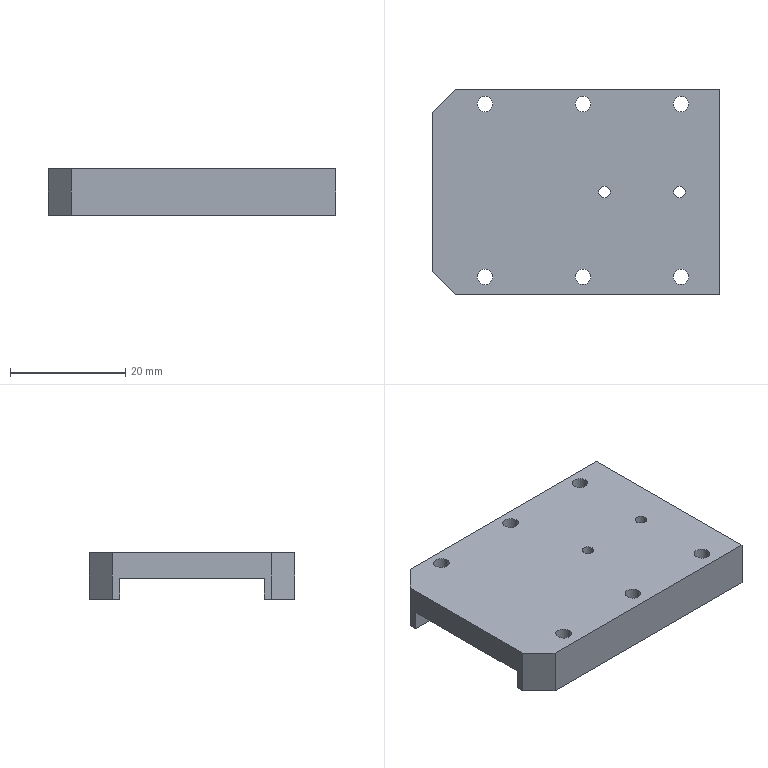Part | SolidWorks | features BaseBody 1 | 1 solid | 28 faces | box 49.9 x 35.6 x 8 mm | volume 9414 mm3 | cylinder 16 | plane 12 | commonest cylinder face diameters 2.7 x12 2 x4
STEP:
#1=CARTESIAN_POINT('',(14.5,0.,-0.5));
#2=VERTEX_POINT('',#1);
#3=CARTESIAN_POINT('',(16.5,0.,-0.5));
#4=VERTEX_POINT('',#3);
#5=CARTESIAN_POINT('',(15.5,0.,-0.5));
#6=DIRECTION('',(0.,0.,1.));
#7=DIRECTION('',(0.,-1.,0.));
#8=AXIS2_PLACEMENT_3D('',#5,#6,#7);
#9=CIRCLE('',#8,1.);
#10=EDGE_CURVE('',#2,#4,#9,.T.);
#11=ORIENTED_EDGE('',*,*,#10,.F.);
#12=CARTESIAN_POINT('',(14.5,0.,4.));
#13=VERTEX_POINT('',#12);
#14=CARTESIAN_POINT('',(14.5,0.,-4.));
#15=DIRECTION('',(0.,0.,1.));
#16=VECTOR('',#15,1000.);
#17=LINE('',#14,#16);
#18=EDGE_CURVE('',#2,#13,#17,.T.);
#19=ORIENTED_EDGE('',*,*,#18,.T.);
#20=CARTESIAN_POINT('',(16.5,0.,4.));
#21=VERTEX_POINT('',#20);
#22=CARTESIAN_POINT('',(15.5,0.,4.));
#23=DIRECTION('',(0.,0.,1.));
#24=DIRECTION('',(1.,0.,0.));
#25=AXIS2_PLACEMENT_3D('',#22,#23,#24);
#26=CIRCLE('',#25,1.);
#27=EDGE_CURVE('',#13,#21,#26,.T.);
#28=ORIENTED_EDGE('',*,*,#27,.T.);
#29=CARTESIAN_POINT('',(16.5,0.,-4.));
#30=DIRECTION('',(0.,0.,1.));
#31=VECTOR('',#30,1000.);
#32=LINE('',#29,#31);
#33=EDGE_CURVE('',#4,#21,#32,.T.);
#34=ORIENTED_EDGE('',*,*,#33,.F.);
#35=EDGE_LOOP('',(#11,#19,#28,#34));
#36=FACE_OUTER_BOUND('',#35,.T.);
#37=CARTESIAN_POINT('',(15.5,0.,-4.));
#38=DIRECTION('',(0.,0.,1.));
#39=DIRECTION('',(1.,0.,0.));
#40=AXIS2_PLACEMENT_3D('',#37,#38,#39);
#41=CYLINDRICAL_SURFACE('',#40,1.);
#42=ADVANCED_FACE('',(#36),#41,.F.);
#43=CARTESIAN_POINT('',(1.5,0.,-0.5));
#44=VERTEX_POINT('',#43);
#45=CARTESIAN_POINT('',(3.5,0.,-0.5));
#46=VERTEX_POINT('',#45);
#47=CARTESIAN_POINT('',(2.5,0.,-0.5));
#48=DIRECTION('',(0.,0.,1.));
#49=DIRECTION('',(0.,-1.,0.));
#50=AXIS2_PLACEMENT_3D('',#47,#48,#49);
#51=CIRCLE('',#50,1.);
#52=EDGE_CURVE('',#44,#46,#51,.T.);
#53=ORIENTED_EDGE('',*,*,#52,.F.);
#54=CARTESIAN_POINT('',(1.5,0.,4.));
#55=VERTEX_POINT('',#54);
#56=CARTESIAN_POINT('',(1.5,0.,-4.));
#57=DIRECTION('',(0.,0.,1.));
#58=VECTOR('',#57,1000.);
#59=LINE('',#56,#58);
#60=EDGE_CURVE('',#44,#55,#59,.T.);
#61=ORIENTED_EDGE('',*,*,#60,.T.);
#62=CARTESIAN_POINT('',(3.5,0.,4.));
#63=VERTEX_POINT('',#62);
#64=CARTESIAN_POINT('',(2.5,0.,4.));
#65=DIRECTION('',(0.,0.,1.));
#66=DIRECTION('',(1.,0.,0.));
#67=AXIS2_PLACEMENT_3D('',#64,#65,#66);
#68=CIRCLE('',#67,1.);
#69=EDGE_CURVE('',#55,#63,#68,.T.);
#70=ORIENTED_EDGE('',*,*,#69,.T.);
#71=CARTESIAN_POINT('',(3.5,0.,-4.));
#72=DIRECTION('',(0.,0.,1.));
#73=VECTOR('',#72,1000.);
#74=LINE('',#71,#73);
#75=EDGE_CURVE('',#46,#63,#74,.T.);
#76=ORIENTED_EDGE('',*,*,#75,.F.);
#77=EDGE_LOOP('',(#53,#61,#70,#76));
#78=FACE_OUTER_BOUND('',#77,.T.);
#79=CARTESIAN_POINT('',(2.5,0.,-4.));
#80=DIRECTION('',(0.,0.,1.));
#81=DIRECTION('',(1.,0.,0.));
#82=AXIS2_PLACEMENT_3D('',#79,#80,#81);
#83=CYLINDRICAL_SURFACE('',#82,1.);
#84=ADVANCED_FACE('',(#78),#83,.F.);
#85=CARTESIAN_POINT('',(17.119,15.267,4.));
#86=VERTEX_POINT('',#85);
#87=CARTESIAN_POINT('',(14.419,15.267,4.));
#88=VERTEX_POINT('',#87);
#89=CARTESIAN_POINT('',(15.769,15.267,4.));
#90=DIRECTION('',(0.,0.,-1.));
#91=DIRECTION('',(-1.,0.,0.));
#92=AXIS2_PLACEMENT_3D('',#89,#90,#91);
#93=CIRCLE('',#92,1.35);
#94=EDGE_CURVE('',#86,#88,#93,.T.);
#95=ORIENTED_EDGE('',*,*,#94,.F.);
#96=CARTESIAN_POINT('',(17.119,15.267,-4.));
#97=VERTEX_POINT('',#96);
#98=CARTESIAN_POINT('',(17.119,15.267,4.));
#99=DIRECTION('',(0.,0.,-1.));
#100=VECTOR('',#99,1000.);
#101=LINE('',#98,#100);
#102=EDGE_CURVE('',#86,#97,#101,.T.);
#103=ORIENTED_EDGE('',*,*,#102,.T.);
#104=CARTESIAN_POINT('',(14.419,15.267,-4.));
#105=VERTEX_POINT('',#104);
#106=CARTESIAN_POINT('',(15.769,15.267,-4.));
#107=DIRECTION('',(0.,0.,-1.));
#108=DIRECTION('',(-1.,0.,0.));
#109=AXIS2_PLACEMENT_3D('',#106,#107,#108);
#110=CIRCLE('',#109,1.35);
#111=EDGE_CURVE('',#97,#105,#110,.T.);
#112=ORIENTED_EDGE('',*,*,#111,.T.);
#113=CARTESIAN_POINT('',(14.419,15.267,4.));
#114=DIRECTION('',(0.,0.,-1.));
#115=VECTOR('',#114,1000.);
#116=LINE('',#113,#115);
#117=EDGE_CURVE('',#88,#105,#116,.T.);
#118=ORIENTED_EDGE('',*,*,#117,.F.);
#119=EDGE_LOOP('',(#95,#103,#112,#118));
#120=FACE_OUTER_BOUND('',#119,.T.);
#121=CARTESIAN_POINT('',(15.769,15.267,4.));
#122=DIRECTION('',(0.,0.,-1.));
#123=DIRECTION('',(-1.,0.,0.));
#124=AXIS2_PLACEMENT_3D('',#121,#122,#123);
#125=CYLINDRICAL_SURFACE('',#124,1.35);
#126=ADVANCED_FACE('',(#120),#125,.F.);
#127=CARTESIAN_POINT('',(0.1194,15.267,4.));
#128=VERTEX_POINT('',#127);
#129=CARTESIAN_POINT('',(-2.581,15.267,4.));
#130=VERTEX_POINT('',#129);
#131=CARTESIAN_POINT('',(-1.231,15.267,4.));
#132=DIRECTION('',(0.,0.,-1.));
#133=DIRECTION('',(-1.,0.,0.));
#134=AXIS2_PLACEMENT_3D('',#131,#132,#133);
#135=CIRCLE('',#134,1.35);
#136=EDGE_CURVE('',#128,#130,#135,.T.);
#137=ORIENTED_EDGE('',*,*,#136,.F.);
#138=CARTESIAN_POINT('',(0.1194,15.267,-4.));
#139=VERTEX_POINT('',#138);
#140=CARTESIAN_POINT('',(0.1194,15.267,4.));
#141=DIRECTION('',(0.,0.,-1.));
#142=VECTOR('',#141,1000.);
#143=LINE('',#140,#142);
#144=EDGE_CURVE('',#128,#139,#143,.T.);
#145=ORIENTED_EDGE('',*,*,#144,.T.);
#146=CARTESIAN_POINT('',(-2.581,15.267,-4.));
#147=VERTEX_POINT('',#146);
#148=CARTESIAN_POINT('',(-1.231,15.267,-4.));
#149=DIRECTION('',(0.,0.,-1.));
#150=DIRECTION('',(-1.,0.,0.));
#151=AXIS2_PLACEMENT_3D('',#148,#149,#150);
#152=CIRCLE('',#151,1.35);
#153=EDGE_CURVE('',#139,#147,#152,.T.);
#154=ORIENTED_EDGE('',*,*,#153,.T.);
#155=CARTESIAN_POINT('',(-2.581,15.267,4.));
#156=DIRECTION('',(0.,0.,-1.));
#157=VECTOR('',#156,1000.);
#158=LINE('',#155,#157);
#159=EDGE_CURVE('',#130,#147,#158,.T.);
#160=ORIENTED_EDGE('',*,*,#159,.F.);
#161=EDGE_LOOP('',(#137,#145,#154,#160));
#162=FACE_OUTER_BOUND('',#161,.T.);
#163=CARTESIAN_POINT('',(-1.231,15.267,4.));
#164=DIRECTION('',(0.,0.,-1.));
#165=DIRECTION('',(-1.,0.,0.));
#166=AXIS2_PLACEMENT_3D('',#163,#164,#165);
#167=CYLINDRICAL_SURFACE('',#166,1.35);
#168=ADVANCED_FACE('',(#162),#167,.F.);
#169=CARTESIAN_POINT('',(-16.881,15.267,4.));
#170=VERTEX_POINT('',#169);
#171=CARTESIAN_POINT('',(-19.581,15.267,4.));
#172=VERTEX_POINT('',#171);
#173=CARTESIAN_POINT('',(-18.231,15.267,4.));
#174=DIRECTION('',(0.,0.,-1.));
#175=DIRECTION('',(-1.,0.,0.));
#176=AXIS2_PLACEMENT_3D('',#173,#174,#175);
#177=CIRCLE('',#176,1.35);
#178=EDGE_CURVE('',#170,#172,#177,.T.);
#179=ORIENTED_EDGE('',*,*,#178,.F.);
#180=CARTESIAN_POINT('',(-16.881,15.267,-4.));
#181=VERTEX_POINT('',#180);
#182=CARTESIAN_POINT('',(-16.881,15.267,4.));
#183=DIRECTION('',(0.,0.,-1.));
#184=VECTOR('',#183,1000.);
#185=LINE('',#182,#184);
#186=EDGE_CURVE('',#170,#181,#185,.T.);
#187=ORIENTED_EDGE('',*,*,#186,.T.);
#188=CARTESIAN_POINT('',(-19.581,15.267,-4.));
#189=VERTEX_POINT('',#188);
#190=CARTESIAN_POINT('',(-18.231,15.267,-4.));
#191=DIRECTION('',(0.,0.,-1.));
#192=DIRECTION('',(-1.,0.,0.));
#193=AXIS2_PLACEMENT_3D('',#190,#191,#192);
#194=CIRCLE('',#193,1.35);
#195=EDGE_CURVE('',#181,#189,#194,.T.);
#196=ORIENTED_EDGE('',*,*,#195,.T.);
#197=CARTESIAN_POINT('',(-19.581,15.267,4.));
#198=DIRECTION('',(0.,0.,-1.));
#199=VECTOR('',#198,1000.);
#200=LINE('',#197,#199);
#201=EDGE_CURVE('',#172,#189,#200,.T.);
#202=ORIENTED_EDGE('',*,*,#201,.F.);
#203=EDGE_LOOP('',(#179,#187,#196,#202));
#204=FACE_OUTER_BOUND('',#203,.T.);
#205=CARTESIAN_POINT('',(-18.231,15.267,4.));
#206=DIRECTION('',(0.,0.,-1.));
#207=DIRECTION('',(-1.,0.,0.));
#208=AXIS2_PLACEMENT_3D('',#205,#206,#207);
#209=CYLINDRICAL_SURFACE('',#208,1.35);
#210=ADVANCED_FACE('',(#204),#209,.F.);
#211=CARTESIAN_POINT('',(-16.881,-14.733,4.));
#212=VERTEX_POINT('',#211);
#213=CARTESIAN_POINT('',(-19.581,-14.733,4.));
#214=VERTEX_POINT('',#213);
#215=CARTESIAN_POINT('',(-18.231,-14.733,4.));
#216=DIRECTION('',(0.,0.,-1.));
#217=DIRECTION('',(-1.,0.,0.));
#218=AXIS2_PLACEMENT_3D('',#215,#216,#217);
#219=CIRCLE('',#218,1.35);
#220=EDGE_CURVE('',#212,#214,#219,.T.);
#221=ORIENTED_EDGE('',*,*,#220,.F.);
#222=CARTESIAN_POINT('',(-16.881,-14.733,-4.));
#223=VERTEX_POINT('',#222);
#224=CARTESIAN_POINT('',(-16.881,-14.733,4.));
#225=DIRECTION('',(0.,0.,-1.));
#226=VECTOR('',#225,1000.);
#227=LINE('',#224,#226);
#228=EDGE_CURVE('',#212,#223,#227,.T.);
#229=ORIENTED_EDGE('',*,*,#228,.T.);
#230=CARTESIAN_POINT('',(-19.581,-14.733,-4.));
#231=VERTEX_POINT('',#230);
#232=CARTESIAN_POINT('',(-18.231,-14.733,-4.));
#233=DIRECTION('',(0.,0.,-1.));
#234=DIRECTION('',(-1.,0.,0.));
#235=AXIS2_PLACEMENT_3D('',#232,#233,#234);
#236=CIRCLE('',#235,1.35);
#237=EDGE_CURVE('',#223,#231,#236,.T.);
#238=ORIENTED_EDGE('',*,*,#237,.T.);
#239=CARTESIAN_POINT('',(-19.581,-14.733,4.));
#240=DIRECTION('',(0.,0.,-1.));
#241=VECTOR('',#240,1000.);
#242=LINE('',#239,#241);
#243=EDGE_CURVE('',#214,#231,#242,.T.);
#244=ORIENTED_EDGE('',*,*,#243,.F.);
#245=EDGE_LOOP('',(#221,#229,#238,#244));
#246=FACE_OUTER_BOUND('',#245,.T.);
#247=CARTESIAN_POINT('',(-18.231,-14.733,4.));
#248=DIRECTION('',(0.,0.,-1.));
#249=DIRECTION('',(-1.,0.,0.));
#250=AXIS2_PLACEMENT_3D('',#247,#248,#249);
#251=CYLINDRICAL_SURFACE('',#250,1.35);
#252=ADVANCED_FACE('',(#246),#251,.F.);
#253=CARTESIAN_POINT('',(0.1194,-14.733,4.));
#254=VERTEX_POINT('',#253);
#255=CARTESIAN_POINT('',(-2.581,-14.733,4.));
#256=VERTEX_POINT('',#255);
#257=CARTESIAN_POINT('',(-1.231,-14.733,4.));
#258=DIRECTION('',(0.,0.,-1.));
#259=DIRECTION('',(-1.,0.,0.));
#260=AXIS2_PLACEMENT_3D('',#257,#258,#259);
#261=CIRCLE('',#260,1.35);
#262=EDGE_CURVE('',#254,#256,#261,.T.);
#263=ORIENTED_EDGE('',*,*,#262,.F.);
#264=CARTESIAN_POINT('',(0.1194,-14.733,-4.));
#265=VERTEX_POINT('',#264);
#266=CARTESIAN_POINT('',(0.1194,-14.733,4.));
#267=DIRECTION('',(0.,0.,-1.));
#268=VECTOR('',#267,1000.);
#269=LINE('',#266,#268);
#270=EDGE_CURVE('',#254,#265,#269,.T.);
#271=ORIENTED_EDGE('',*,*,#270,.T.);
#272=CARTESIAN_POINT('',(-2.581,-14.733,-4.));
#273=VERTEX_POINT('',#272);
#274=CARTESIAN_POINT('',(-1.231,-14.733,-4.));
#275=DIRECTION('',(0.,0.,-1.));
#276=DIRECTION('',(-1.,0.,0.));
#277=AXIS2_PLACEMENT_3D('',#274,#275,#276);
#278=CIRCLE('',#277,1.35);
#279=EDGE_CURVE('',#265,#273,#278,.T.);
#280=ORIENTED_EDGE('',*,*,#279,.T.);
#281=CARTESIAN_POINT('',(-2.581,-14.733,4.));
#282=DIRECTION('',(0.,0.,-1.));
#283=VECTOR('',#282,1000.);
#284=LINE('',#281,#283);
#285=EDGE_CURVE('',#256,#273,#284,.T.);
#286=ORIENTED_EDGE('',*,*,#285,.F.);
#287=EDGE_LOOP('',(#263,#271,#280,#286));
#288=FACE_OUTER_BOUND('',#287,.T.);
#289=CARTESIAN_POINT('',(-1.231,-14.733,4.));
#290=DIRECTION('',(0.,0.,-1.));
#291=DIRECTION('',(-1.,0.,0.));
#292=AXIS2_PLACEMENT_3D('',#289,#290,#291);
#293=CYLINDRICAL_SURFACE('',#292,1.35);
#294=ADVANCED_FACE('',(#288),#293,.F.);
#295=CARTESIAN_POINT('',(17.119,-14.733,4.));
#296=VERTEX_POINT('',#295);
#297=CARTESIAN_POINT('',(14.419,-14.733,4.));
#298=VERTEX_POINT('',#297);
#299=CARTESIAN_POINT('',(15.769,-14.733,4.));
#300=DIRECTION('',(0.,0.,-1.));
#301=DIRECTION('',(-1.,0.,0.));
#302=AXIS2_PLACEMENT_3D('',#299,#300,#301);
#303=CIRCLE('',#302,1.35);
#304=EDGE_CURVE('',#296,#298,#303,.T.);
#305=ORIENTED_EDGE('',*,*,#304,.F.);
#306=CARTESIAN_POINT('',(17.119,-14.733,-4.));
#307=VERTEX_POINT('',#306);
#308=CARTESIAN_POINT('',(17.119,-14.733,4.));
#309=DIRECTION('',(0.,0.,-1.));
#310=VECTOR('',#309,1000.);
#311=LINE('',#308,#310);
#312=EDGE_CURVE('',#296,#307,#311,.T.);
#313=ORIENTED_EDGE('',*,*,#312,.T.);
#314=CARTESIAN_POINT('',(14.419,-14.733,-4.));
#315=VERTEX_POINT('',#314);
#316=CARTESIAN_POINT('',(15.769,-14.733,-4.));
#317=DIRECTION('',(0.,0.,-1.));
#318=DIRECTION('',(-1.,0.,0.));
#319=AXIS2_PLACEMENT_3D('',#316,#317,#318);
#320=CIRCLE('',#319,1.35);
#321=EDGE_CURVE('',#307,#315,#320,.T.);
#322=ORIENTED_EDGE('',*,*,#321,.T.);
#323=CARTESIAN_POINT('',(14.419,-14.733,4.));
#324=DIRECTION('',(0.,0.,-1.));
#325=VECTOR('',#324,1000.);
#326=LINE('',#323,#325);
#327=EDGE_CURVE('',#298,#315,#326,.T.);
#328=ORIENTED_EDGE('',*,*,#327,.F.);
#329=EDGE_LOOP('',(#305,#313,#322,#328));
#330=FACE_OUTER_BOUND('',#329,.T.);
#331=CARTESIAN_POINT('',(15.769,-14.733,4.));
#332=DIRECTION('',(0.,0.,-1.));
#333=DIRECTION('',(-1.,0.,0.));
#334=AXIS2_PLACEMENT_3D('',#331,#332,#333);
#335=CYLINDRICAL_SURFACE('',#334,1.35);
#336=ADVANCED_FACE('',(#330),#335,.F.);
#337=CARTESIAN_POINT('',(22.5,12.5,-4.));
#338=VERTEX_POINT('',#337);
#339=CARTESIAN_POINT('',(-27.4,12.5,-4.));
#340=VERTEX_POINT('',#339);
#341=CARTESIAN_POINT('',(22.5,12.5,-4.));
#342=DIRECTION('',(-1.,0.,0.));
#343=VECTOR('',#342,1000.);
#344=LINE('',#341,#343);
#345=EDGE_CURVE('',#338,#340,#344,.T.);
#346=ORIENTED_EDGE('',*,*,#345,.T.);
#347=CARTESIAN_POINT('',(-27.4,13.8,-4.));
#348=VERTEX_POINT('',#347);
#349=CARTESIAN_POINT('',(-27.4,17.8,-4.));
#350=DIRECTION('',(0.,1.,0.));
#351=VECTOR('',#350,1000.);
#352=LINE('',#349,#351);
#353=EDGE_CURVE('',#340,#348,#352,.T.);
#354=ORIENTED_EDGE('',*,*,#353,.T.);
#355=CARTESIAN_POINT('',(-23.4,17.8,-4.));
#356=VERTEX_POINT('',#355);
#357=CARTESIAN_POINT('',(-20.6,20.6,-4.));
#358=DIRECTION('',(0.7071,0.7071,0.));
#359=VECTOR('',#358,1000.);
#360=LINE('',#357,#359);
#361=EDGE_CURVE('',#348,#356,#360,.T.);
#362=ORIENTED_EDGE('',*,*,#361,.T.);
#363=CARTESIAN_POINT('',(22.5,17.8,-4.));
#364=VERTEX_POINT('',#363);
#365=CARTESIAN_POINT('',(22.5,17.8,-4.));
#366=DIRECTION('',(-1.,0.,0.));
#367=VECTOR('',#366,1000.);
#368=LINE('',#365,#367);
#369=EDGE_CURVE('',#364,#356,#368,.T.);
#370=ORIENTED_EDGE('',*,*,#369,.F.);
#371=CARTESIAN_POINT('',(22.5,17.8,-4.));
#372=DIRECTION('',(0.,1.,0.));
#373=VECTOR('',#372,1000.);
#374=LINE('',#371,#373);
#375=EDGE_CURVE('',#338,#364,#374,.T.);
#376=ORIENTED_EDGE('',*,*,#375,.F.);
#377=EDGE_LOOP('',(#346,#354,#362,#370,#376));
#378=FACE_OUTER_BOUND('',#377,.T.);
#379=CARTESIAN_POINT('',(-18.231,15.267,-4.));
#380=DIRECTION('',(0.,0.,-1.));
#381=DIRECTION('',(-1.,0.,0.));
#382=AXIS2_PLACEMENT_3D('',#379,#380,#381);
#383=CIRCLE('',#382,1.35);
#384=EDGE_CURVE('',#189,#181,#383,.T.);
#385=ORIENTED_EDGE('',*,*,#384,.F.);
#386=ORIENTED_EDGE('',*,*,#195,.F.);
#387=EDGE_LOOP('',(#385,#386));
#388=FACE_BOUND('',#387,.T.);
#389=CARTESIAN_POINT('',(-1.231,15.267,-4.));
#390=DIRECTION('',(0.,0.,-1.));
#391=DIRECTION('',(-1.,0.,0.));
#392=AXIS2_PLACEMENT_3D('',#389,#390,#391);
#393=CIRCLE('',#392,1.35);
#394=EDGE_CURVE('',#147,#139,#393,.T.);
#395=ORIENTED_EDGE('',*,*,#394,.F.);
#396=ORIENTED_EDGE('',*,*,#153,.F.);
#397=EDGE_LOOP('',(#395,#396));
#398=FACE_BOUND('',#397,.T.);
#399=CARTESIAN_POINT('',(15.769,15.267,-4.));
#400=DIRECTION('',(0.,0.,-1.));
#401=DIRECTION('',(-1.,0.,0.));
#402=AXIS2_PLACEMENT_3D('',#399,#400,#401);
#403=CIRCLE('',#402,1.35);
#404=EDGE_CURVE('',#105,#97,#403,.T.);
#405=ORIENTED_EDGE('',*,*,#404,.F.);
#406=ORIENTED_EDGE('',*,*,#111,.F.);
#407=EDGE_LOOP('',(#405,#406));
#408=FACE_BOUND('',#407,.T.);
#409=CARTESIAN_POINT('',(0.,0.,-4.));
#410=DIRECTION('',(0.,0.,-1.));
#411=DIRECTION('',(-1.,0.,0.));
#412=AXIS2_PLACEMENT_3D('',#409,#410,#411);
#413=PLANE('',#412);
#414=ADVANCED_FACE('',(#378,#388,#398,#408),#413,.T.);
#415=CARTESIAN_POINT('',(-23.4,-17.8,4.));
#416=VERTEX_POINT('',#415);
#417=CARTESIAN_POINT('',(22.5,-17.8,4.));
#418=VERTEX_POINT('',#417);
#419=CARTESIAN_POINT('',(22.5,-17.8,4.));
#420=DIRECTION('',(1.,0.,0.));
#421=VECTOR('',#420,1000.);
#422=LINE('',#419,#421);
#423=EDGE_CURVE('',#416,#418,#422,.T.);
#424=ORIENTED_EDGE('',*,*,#423,.F.);
#425=CARTESIAN_POINT('',(-23.4,-17.8,-4.));
#426=VERTEX_POINT('',#425);
#427=CARTESIAN_POINT('',(-23.4,-17.8,-4.));
#428=DIRECTION('',(0.,0.,-1.));
#429=VECTOR('',#428,1000.);
#430=LINE('',#427,#429);
#431=EDGE_CURVE('',#416,#426,#430,.T.);
#432=ORIENTED_EDGE('',*,*,#431,.T.);
#433=CARTESIAN_POINT('',(22.5,-17.8,-4.));
#434=VERTEX_POINT('',#433);
#435=CARTESIAN_POINT('',(22.5,-17.8,-4.));
#436=DIRECTION('',(1.,0.,0.));
#437=VECTOR('',#436,1000.);
#438=LINE('',#435,#437);
#439=EDGE_CURVE('',#426,#434,#438,.T.);
#440=ORIENTED_EDGE('',*,*,#439,.T.);
#441=CARTESIAN_POINT('',(22.5,-17.8,4.));
#442=DIRECTION('',(0.,0.,-1.));
#443=VECTOR('',#442,1000.);
#444=LINE('',#441,#443);
#445=EDGE_CURVE('',#418,#434,#444,.T.);
#446=ORIENTED_EDGE('',*,*,#445,.F.);
#447=EDGE_LOOP('',(#424,#432,#440,#446));
#448=FACE_OUTER_BOUND('',#447,.T.);
#449=CARTESIAN_POINT('',(22.5,-17.8,4.));
#450=DIRECTION('',(0.,1.,0.));
#451=DIRECTION('',(-1.,0.,0.));
#452=AXIS2_PLACEMENT_3D('',#449,#450,#451);
#453=PLANE('',#452);
#454=ADVANCED_FACE('',(#448),#453,.F.);
#455=CARTESIAN_POINT('',(22.5,-12.5,-0.5));
#456=VERTEX_POINT('',#455);
#457=CARTESIAN_POINT('',(22.5,12.5,-0.5));
#458=VERTEX_POINT('',#457);
#459=CARTESIAN_POINT('',(22.5,12.5,-0.5));
#460=DIRECTION('',(0.,1.,0.));
#461=VECTOR('',#460,1000.);
#462=LINE('',#459,#461);
#463=EDGE_CURVE('',#456,#458,#462,.T.);
#464=ORIENTED_EDGE('',*,*,#463,.T.);
#465=CARTESIAN_POINT('',(22.5,12.5,-0.5));
#466=DIRECTION('',(0.,0.,-1.));
#467=VECTOR('',#466,1000.);
#468=LINE('',#465,#467);
#469=EDGE_CURVE('',#458,#338,#468,.T.);
#470=ORIENTED_EDGE('',*,*,#469,.T.);
#471=ORIENTED_EDGE('',*,*,#375,.T.);
#472=CARTESIAN_POINT('',(22.5,17.8,4.));
#473=VERTEX_POINT('',#472);
#474=CARTESIAN_POINT('',(22.5,17.8,4.));
#475=DIRECTION('',(0.,0.,-1.));
#476=VECTOR('',#475,1000.);
#477=LINE('',#474,#476);
#478=EDGE_CURVE('',#473,#364,#477,.T.);
#479=ORIENTED_EDGE('',*,*,#478,.F.);
#480=CARTESIAN_POINT('',(22.5,17.8,4.));
#481=DIRECTION('',(0.,1.,0.));
#482=VECTOR('',#481,1000.);
#483=LINE('',#480,#482);
#484=EDGE_CURVE('',#418,#473,#483,.T.);
#485=ORIENTED_EDGE('',*,*,#484,.F.);
#486=ORIENTED_EDGE('',*,*,#445,.T.);
#487=CARTESIAN_POINT('',(22.5,-12.5,-4.));
#488=VERTEX_POINT('',#487);
#489=CARTESIAN_POINT('',(22.5,17.8,-4.));
#490=DIRECTION('',(0.,1.,0.));
#491=VECTOR('',#490,1000.);
#492=LINE('',#489,#491);
#493=EDGE_CURVE('',#434,#488,#492,.T.);
#494=ORIENTED_EDGE('',*,*,#493,.T.);
#495=CARTESIAN_POINT('',(22.5,-12.5,-0.5));
#496=DIRECTION('',(0.,0.,1.));
#497=VECTOR('',#496,1000.);
#498=LINE('',#495,#497);
#499=EDGE_CURVE('',#488,#456,#498,.T.);
#500=ORIENTED_EDGE('',*,*,#499,.T.);
#501=EDGE_LOOP('',(#464,#470,#471,#479,#485,#486,#494,#500));
#502=FACE_OUTER_BOUND('',#501,.T.);
#503=CARTESIAN_POINT('',(22.5,17.8,4.));
#504=DIRECTION('',(-1.,0.,0.));
#505=DIRECTION('',(0.,0.,1.));
#506=AXIS2_PLACEMENT_3D('',#503,#504,#505);
#507=PLANE('',#506);
#508=ADVANCED_FACE('',(#502),#507,.F.);
#509=ORIENTED_EDGE('',*,*,#369,.T.);
#510=CARTESIAN_POINT('',(-23.4,17.8,4.));
#511=VERTEX_POINT('',#510);
#512=CARTESIAN_POINT('',(-23.4,17.8,4.));
#513=DIRECTION('',(0.,0.,1.));
#514=VECTOR('',#513,1000.);
#515=LINE('',#512,#514);
#516=EDGE_CURVE('',#356,#511,#515,.T.);
#517=ORIENTED_EDGE('',*,*,#516,.T.);
#518=CARTESIAN_POINT('',(22.5,17.8,4.));
#519=DIRECTION('',(-1.,0.,0.));
#520=VECTOR('',#519,1000.);
#521=LINE('',#518,#520);
#522=EDGE_CURVE('',#473,#511,#521,.T.);
#523=ORIENTED_EDGE('',*,*,#522,.F.);
#524=ORIENTED_EDGE('',*,*,#478,.T.);
#525=EDGE_LOOP('',(#509,#517,#523,#524));
#526=FACE_OUTER_BOUND('',#525,.T.);
#527=CARTESIAN_POINT('',(22.5,17.8,4.));
#528=DIRECTION('',(0.,-1.,0.));
#529=DIRECTION('',(1.,0.,0.));
#530=AXIS2_PLACEMENT_3D('',#527,#528,#529);
#531=PLANE('',#530);
#532=ADVANCED_FACE('',(#526),#531,.F.);
#533=CARTESIAN_POINT('',(15.5,0.,4.));
#534=DIRECTION('',(0.,0.,1.));
#535=DIRECTION('',(1.,0.,0.));
#536=AXIS2_PLACEMENT_3D('',#533,#534,#535);
#537=CIRCLE('',#536,1.);
#538=EDGE_CURVE('',#21,#13,#537,.T.);
#539=ORIENTED_EDGE('',*,*,#538,.F.);
#540=ORIENTED_EDGE('',*,*,#27,.F.);
#541=EDGE_LOOP('',(#539,#540));
#542=FACE_BOUND('',#541,.T.);
#543=CARTESIAN_POINT('',(2.5,0.,4.));
#544=DIRECTION('',(0.,0.,1.));
#545=DIRECTION('',(1.,0.,0.));
#546=AXIS2_PLACEMENT_3D('',#543,#544,#545);
#547=CIRCLE('',#546,1.);
#548=EDGE_CURVE('',#63,#55,#547,.T.);
#549=ORIENTED_EDGE('',*,*,#548,.F.);
#550=ORIENTED_EDGE('',*,*,#69,.F.);
#551=EDGE_LOOP('',(#549,#550));
#552=FACE_BOUND('',#551,.T.);
#553=CARTESIAN_POINT('',(15.769,15.267,4.));
#554=DIRECTION('',(0.,0.,-1.));
#555=DIRECTION('',(-1.,0.,0.));
#556=AXIS2_PLACEMENT_3D('',#553,#554,#555);
#557=CIRCLE('',#556,1.35);
#558=EDGE_CURVE('',#88,#86,#557,.T.);
#559=ORIENTED_EDGE('',*,*,#558,.T.);
#560=ORIENTED_EDGE('',*,*,#94,.T.);
#561=EDGE_LOOP('',(#559,#560));
#562=FACE_BOUND('',#561,.T.);
#563=CARTESIAN_POINT('',(-1.231,15.267,4.));
#564=DIRECTION('',(0.,0.,-1.));
#565=DIRECTION('',(-1.,0.,0.));
#566=AXIS2_PLACEMENT_3D('',#563,#564,#565);
#567=CIRCLE('',#566,1.35);
#568=EDGE_CURVE('',#130,#128,#567,.T.);
#569=ORIENTED_EDGE('',*,*,#568,.T.);
#570=ORIENTED_EDGE('',*,*,#136,.T.);
#571=EDGE_LOOP('',(#569,#570));
#572=FACE_BOUND('',#571,.T.);
#573=CARTESIAN_POINT('',(-18.231,15.267,4.));
#574=DIRECTION('',(0.,0.,-1.));
#575=DIRECTION('',(-1.,0.,0.));
#576=AXIS2_PLACEMENT_3D('',#573,#574,#575);
#577=CIRCLE('',#576,1.35);
#578=EDGE_CURVE('',#172,#170,#577,.T.);
#579=ORIENTED_EDGE('',*,*,#578,.T.);
#580=ORIENTED_EDGE('',*,*,#178,.T.);
#581=EDGE_LOOP('',(#579,#580));
#582=FACE_BOUND('',#581,.T.);
#583=CARTESIAN_POINT('',(-18.231,-14.733,4.));
#584=DIRECTION('',(0.,0.,-1.));
#585=DIRECTION('',(-1.,0.,0.));
#586=AXIS2_PLACEMENT_3D('',#583,#584,#585);
#587=CIRCLE('',#586,1.35);
#588=EDGE_CURVE('',#214,#212,#587,.T.);
#589=ORIENTED_EDGE('',*,*,#588,.T.);
#590=ORIENTED_EDGE('',*,*,#220,.T.);
#591=EDGE_LOOP('',(#589,#590));
#592=FACE_BOUND('',#591,.T.);
#593=CARTESIAN_POINT('',(-1.231,-14.733,4.));
#594=DIRECTION('',(0.,0.,-1.));
#595=DIRECTION('',(-1.,0.,0.));
#596=AXIS2_PLACEMENT_3D('',#593,#594,#595);
#597=CIRCLE('',#596,1.35);
#598=EDGE_CURVE('',#256,#254,#597,.T.);
#599=ORIENTED_EDGE('',*,*,#598,.T.);
#600=ORIENTED_EDGE('',*,*,#262,.T.);
#601=EDGE_LOOP('',(#599,#600));
#602=FACE_BOUND('',#601,.T.);
#603=CARTESIAN_POINT('',(15.769,-14.733,4.));
#604=DIRECTION('',(0.,0.,-1.));
#605=DIRECTION('',(-1.,0.,0.));
#606=AXIS2_PLACEMENT_3D('',#603,#604,#605);
#607=CIRCLE('',#606,1.35);
#608=EDGE_CURVE('',#298,#296,#607,.T.);
#609=ORIENTED_EDGE('',*,*,#608,.T.);
#610=ORIENTED_EDGE('',*,*,#304,.T.);
#611=EDGE_LOOP('',(#609,#610));
#612=FACE_BOUND('',#611,.T.);
#613=ORIENTED_EDGE('',*,*,#522,.T.);
#614=CARTESIAN_POINT('',(-27.4,13.8,4.));
#615=VERTEX_POINT('',#614);
#616=CARTESIAN_POINT('',(-27.4,13.8,4.));
#617=DIRECTION('',(-0.7071,-0.7071,0.));
#618=VECTOR('',#617,1000.);
#619=LINE('',#616,#618);
#620=EDGE_CURVE('',#511,#615,#619,.T.);
#621=ORIENTED_EDGE('',*,*,#620,.T.);
#622=CARTESIAN_POINT('',(-27.4,-13.8,4.));
#623=VERTEX_POINT('',#622);
#624=CARTESIAN_POINT('',(-27.4,17.8,4.));
#625=DIRECTION('',(0.,-1.,0.));
#626=VECTOR('',#625,1000.);
#627=LINE('',#624,#626);
#628=EDGE_CURVE('',#615,#623,#627,.T.);
#629=ORIENTED_EDGE('',*,*,#628,.T.);
#630=CARTESIAN_POINT('',(-23.4,-17.8,4.));
#631=DIRECTION('',(0.7071,-0.7071,0.));
#632=VECTOR('',#631,1000.);
#633=LINE('',#630,#632);
#634=EDGE_CURVE('',#623,#416,#633,.T.);
#635=ORIENTED_EDGE('',*,*,#634,.T.);
#636=ORIENTED_EDGE('',*,*,#423,.T.);
#637=ORIENTED_EDGE('',*,*,#484,.T.);
#638=EDGE_LOOP('',(#613,#621,#629,#635,#636,#637));
#639=FACE_OUTER_BOUND('',#638,.T.);
#640=CARTESIAN_POINT('',(0.,0.,4.));
#641=DIRECTION('',(0.,0.,-1.));
#642=DIRECTION('',(-1.,0.,0.));
#643=AXIS2_PLACEMENT_3D('',#640,#641,#642);
#644=PLANE('',#643);
#645=ADVANCED_FACE('',(#542,#552,#562,#572,#582,#592,#602,#612,#639),#644,.F.);
#646=CARTESIAN_POINT('',(-27.4,-12.5,-4.));
#647=VERTEX_POINT('',#646);
#648=CARTESIAN_POINT('',(22.5,-12.5,-4.));
#649=DIRECTION('',(-1.,0.,0.));
#650=VECTOR('',#649,1000.);
#651=LINE('',#648,#650);
#652=EDGE_CURVE('',#488,#647,#651,.T.);
#653=ORIENTED_EDGE('',*,*,#652,.F.);
#654=ORIENTED_EDGE('',*,*,#493,.F.);
#655=ORIENTED_EDGE('',*,*,#439,.F.);
#656=CARTESIAN_POINT('',(-27.4,-13.8,-4.));
#657=VERTEX_POINT('',#656);
#658=CARTESIAN_POINT('',(-20.6,-20.6,-4.));
#659=DIRECTION('',(-0.7071,0.7071,0.));
#660=VECTOR('',#659,1000.);
#661=LINE('',#658,#660);
#662=EDGE_CURVE('',#426,#657,#661,.T.);
#663=ORIENTED_EDGE('',*,*,#662,.T.);
#664=CARTESIAN_POINT('',(-27.4,17.8,-4.));
#665=DIRECTION('',(0.,1.,0.));
#666=VECTOR('',#665,1000.);
#667=LINE('',#664,#666);
#668=EDGE_CURVE('',#657,#647,#667,.T.);
#669=ORIENTED_EDGE('',*,*,#668,.T.);
#670=EDGE_LOOP('',(#653,#654,#655,#663,#669));
#671=FACE_OUTER_BOUND('',#670,.T.);
#672=CARTESIAN_POINT('',(-18.231,-14.733,-4.));
#673=DIRECTION('',(0.,0.,-1.));
#674=DIRECTION('',(-1.,0.,0.));
#675=AXIS2_PLACEMENT_3D('',#672,#673,#674);
#676=CIRCLE('',#675,1.35);
#677=EDGE_CURVE('',#231,#223,#676,.T.);
#678=ORIENTED_EDGE('',*,*,#677,.F.);
#679=ORIENTED_EDGE('',*,*,#237,.F.);
#680=EDGE_LOOP('',(#678,#679));
#681=FACE_BOUND('',#680,.T.);
#682=CARTESIAN_POINT('',(-1.231,-14.733,-4.));
#683=DIRECTION('',(0.,0.,-1.));
#684=DIRECTION('',(-1.,0.,0.));
#685=AXIS2_PLACEMENT_3D('',#682,#683,#684);
#686=CIRCLE('',#685,1.35);
#687=EDGE_CURVE('',#273,#265,#686,.T.);
#688=ORIENTED_EDGE('',*,*,#687,.F.);
#689=ORIENTED_EDGE('',*,*,#279,.F.);
#690=EDGE_LOOP('',(#688,#689));
#691=FACE_BOUND('',#690,.T.);
#692=CARTESIAN_POINT('',(15.769,-14.733,-4.));
#693=DIRECTION('',(0.,0.,-1.));
#694=DIRECTION('',(-1.,0.,0.));
#695=AXIS2_PLACEMENT_3D('',#692,#693,#694);
#696=CIRCLE('',#695,1.35);
#697=EDGE_CURVE('',#315,#307,#696,.T.);
#698=ORIENTED_EDGE('',*,*,#697,.F.);
#699=ORIENTED_EDGE('',*,*,#321,.F.);
#700=EDGE_LOOP('',(#698,#699));
#701=FACE_BOUND('',#700,.T.);
#702=CARTESIAN_POINT('',(0.,0.,-4.));
#703=DIRECTION('',(0.,0.,-1.));
#704=DIRECTION('',(-1.,0.,0.));
#705=AXIS2_PLACEMENT_3D('',#702,#703,#704);
#706=PLANE('',#705);
#707=ADVANCED_FACE('',(#671,#681,#691,#701),#706,.T.);
#708=ORIENTED_EDGE('',*,*,#312,.F.);
#709=ORIENTED_EDGE('',*,*,#608,.F.);
#710=ORIENTED_EDGE('',*,*,#327,.T.);
#711=ORIENTED_EDGE('',*,*,#697,.T.);
#712=EDGE_LOOP('',(#708,#709,#710,#711));
#713=FACE_OUTER_BOUND('',#712,.T.);
#714=CARTESIAN_POINT('',(15.769,-14.733,4.));
#715=DIRECTION('',(0.,0.,-1.));
#716=DIRECTION('',(-1.,0.,0.));
#717=AXIS2_PLACEMENT_3D('',#714,#715,#716);
#718=CYLINDRICAL_SURFACE('',#717,1.35);
#719=ADVANCED_FACE('',(#713),#718,.F.);
#720=ORIENTED_EDGE('',*,*,#270,.F.);
#721=ORIENTED_EDGE('',*,*,#598,.F.);
#722=ORIENTED_EDGE('',*,*,#285,.T.);
#723=ORIENTED_EDGE('',*,*,#687,.T.);
#724=EDGE_LOOP('',(#720,#721,#722,#723));
#725=FACE_OUTER_BOUND('',#724,.T.);
#726=CARTESIAN_POINT('',(-1.231,-14.733,4.));
#727=DIRECTION('',(0.,0.,-1.));
#728=DIRECTION('',(-1.,0.,0.));
#729=AXIS2_PLACEMENT_3D('',#726,#727,#728);
#730=CYLINDRICAL_SURFACE('',#729,1.35);
#731=ADVANCED_FACE('',(#725),#730,.F.);
#732=ORIENTED_EDGE('',*,*,#228,.F.);
#733=ORIENTED_EDGE('',*,*,#588,.F.);
#734=ORIENTED_EDGE('',*,*,#243,.T.);
#735=ORIENTED_EDGE('',*,*,#677,.T.);
#736=EDGE_LOOP('',(#732,#733,#734,#735));
#737=FACE_OUTER_BOUND('',#736,.T.);
#738=CARTESIAN_POINT('',(-18.231,-14.733,4.));
#739=DIRECTION('',(0.,0.,-1.));
#740=DIRECTION('',(-1.,0.,0.));
#741=AXIS2_PLACEMENT_3D('',#738,#739,#740);
#742=CYLINDRICAL_SURFACE('',#741,1.35);
#743=ADVANCED_FACE('',(#737),#742,.F.);
#744=ORIENTED_EDGE('',*,*,#186,.F.);
#745=ORIENTED_EDGE('',*,*,#578,.F.);
#746=ORIENTED_EDGE('',*,*,#201,.T.);
#747=ORIENTED_EDGE('',*,*,#384,.T.);
#748=EDGE_LOOP('',(#744,#745,#746,#747));
#749=FACE_OUTER_BOUND('',#748,.T.);
#750=CARTESIAN_POINT('',(-18.231,15.267,4.));
#751=DIRECTION('',(0.,0.,-1.));
#752=DIRECTION('',(-1.,0.,0.));
#753=AXIS2_PLACEMENT_3D('',#750,#751,#752);
#754=CYLINDRICAL_SURFACE('',#753,1.35);
#755=ADVANCED_FACE('',(#749),#754,.F.);
#756=ORIENTED_EDGE('',*,*,#144,.F.);
#757=ORIENTED_EDGE('',*,*,#568,.F.);
#758=ORIENTED_EDGE('',*,*,#159,.T.);
#759=ORIENTED_EDGE('',*,*,#394,.T.);
#760=EDGE_LOOP('',(#756,#757,#758,#759));
#761=FACE_OUTER_BOUND('',#760,.T.);
#762=CARTESIAN_POINT('',(-1.231,15.267,4.));
#763=DIRECTION('',(0.,0.,-1.));
#764=DIRECTION('',(-1.,0.,0.));
#765=AXIS2_PLACEMENT_3D('',#762,#763,#764);
#766=CYLINDRICAL_SURFACE('',#765,1.35);
#767=ADVANCED_FACE('',(#761),#766,.F.);
#768=ORIENTED_EDGE('',*,*,#102,.F.);
#769=ORIENTED_EDGE('',*,*,#558,.F.);
#770=ORIENTED_EDGE('',*,*,#117,.T.);
#771=ORIENTED_EDGE('',*,*,#404,.T.);
#772=EDGE_LOOP('',(#768,#769,#770,#771));
#773=FACE_OUTER_BOUND('',#772,.T.);
#774=CARTESIAN_POINT('',(15.769,15.267,4.));
#775=DIRECTION('',(0.,0.,-1.));
#776=DIRECTION('',(-1.,0.,0.));
#777=AXIS2_PLACEMENT_3D('',#774,#775,#776);
#778=CYLINDRICAL_SURFACE('',#777,1.35);
#779=ADVANCED_FACE('',(#773),#778,.F.);
#780=CARTESIAN_POINT('',(-27.4,12.5,-0.5));
#781=VERTEX_POINT('',#780);
#782=CARTESIAN_POINT('',(-27.4,12.5,-0.5));
#783=DIRECTION('',(0.,0.,-1.));
#784=VECTOR('',#783,1000.);
#785=LINE('',#782,#784);
#786=EDGE_CURVE('',#781,#340,#785,.T.);
#787=ORIENTED_EDGE('',*,*,#786,.F.);
#788=CARTESIAN_POINT('',(-27.4,-12.5,-0.5));
#789=VERTEX_POINT('',#788);
#790=CARTESIAN_POINT('',(-27.4,12.5,-0.5));
#791=DIRECTION('',(0.,1.,0.));
#792=VECTOR('',#791,1000.);
#793=LINE('',#790,#792);
#794=EDGE_CURVE('',#789,#781,#793,.T.);
#795=ORIENTED_EDGE('',*,*,#794,.F.);
#796=CARTESIAN_POINT('',(-27.4,-12.5,-0.5));
#797=DIRECTION('',(0.,0.,1.));
#798=VECTOR('',#797,1000.);
#799=LINE('',#796,#798);
#800=EDGE_CURVE('',#647,#789,#799,.T.);
#801=ORIENTED_EDGE('',*,*,#800,.F.);
#802=ORIENTED_EDGE('',*,*,#668,.F.);
#803=CARTESIAN_POINT('',(-27.4,-13.8,4.));
#804=DIRECTION('',(0.,0.,1.));
#805=VECTOR('',#804,1000.);
#806=LINE('',#803,#805);
#807=EDGE_CURVE('',#657,#623,#806,.T.);
#808=ORIENTED_EDGE('',*,*,#807,.T.);
#809=ORIENTED_EDGE('',*,*,#628,.F.);
#810=CARTESIAN_POINT('',(-27.4,13.8,-4.));
#811=DIRECTION('',(0.,0.,-1.));
#812=VECTOR('',#811,1000.);
#813=LINE('',#810,#812);
#814=EDGE_CURVE('',#615,#348,#813,.T.);
#815=ORIENTED_EDGE('',*,*,#814,.T.);
#816=ORIENTED_EDGE('',*,*,#353,.F.);
#817=EDGE_LOOP('',(#787,#795,#801,#802,#808,#809,#815,#816));
#818=FACE_OUTER_BOUND('',#817,.T.);
#819=CARTESIAN_POINT('',(-27.4,17.8,39.936));
#820=DIRECTION('',(-1.,0.,0.));
#821=DIRECTION('',(0.,-1.,0.));
#822=AXIS2_PLACEMENT_3D('',#819,#820,#821);
#823=PLANE('',#822);
#824=ADVANCED_FACE('',(#818),#823,.T.);
#825=ORIENTED_EDGE('',*,*,#620,.F.);
#826=ORIENTED_EDGE('',*,*,#516,.F.);
#827=ORIENTED_EDGE('',*,*,#361,.F.);
#828=ORIENTED_EDGE('',*,*,#814,.F.);
#829=EDGE_LOOP('',(#825,#826,#827,#828));
#830=FACE_OUTER_BOUND('',#829,.T.);
#831=CARTESIAN_POINT('',(-27.4,13.8,39.936));
#832=DIRECTION('',(-0.7071,0.7071,0.));
#833=DIRECTION('',(0.,0.,1.));
#834=AXIS2_PLACEMENT_3D('',#831,#832,#833);
#835=PLANE('',#834);
#836=ADVANCED_FACE('',(#830),#835,.T.);
#837=ORIENTED_EDGE('',*,*,#634,.F.);
#838=ORIENTED_EDGE('',*,*,#807,.F.);
#839=ORIENTED_EDGE('',*,*,#662,.F.);
#840=ORIENTED_EDGE('',*,*,#431,.F.);
#841=EDGE_LOOP('',(#837,#838,#839,#840));
#842=FACE_OUTER_BOUND('',#841,.T.);
#843=CARTESIAN_POINT('',(-23.4,-17.8,4.));
#844=DIRECTION('',(-0.7071,-0.7071,0.));
#845=DIRECTION('',(0.,0.,1.));
#846=AXIS2_PLACEMENT_3D('',#843,#844,#845);
#847=PLANE('',#846);
#848=ADVANCED_FACE('',(#842),#847,.T.);
#849=ORIENTED_EDGE('',*,*,#786,.T.);
#850=ORIENTED_EDGE('',*,*,#345,.F.);
#851=ORIENTED_EDGE('',*,*,#469,.F.);
#852=CARTESIAN_POINT('',(22.5,12.5,-0.5));
#853=DIRECTION('',(-1.,0.,0.));
#854=VECTOR('',#853,1000.);
#855=LINE('',#852,#854);
#856=EDGE_CURVE('',#458,#781,#855,.T.);
#857=ORIENTED_EDGE('',*,*,#856,.T.);
#858=EDGE_LOOP('',(#849,#850,#851,#857));
#859=FACE_OUTER_BOUND('',#858,.T.);
#860=CARTESIAN_POINT('',(22.5,12.5,-0.5));
#861=DIRECTION('',(0.,1.,0.));
#862=DIRECTION('',(-1.,0.,0.));
#863=AXIS2_PLACEMENT_3D('',#860,#861,#862);
#864=PLANE('',#863);
#865=ADVANCED_FACE('',(#859),#864,.F.);
#866=CARTESIAN_POINT('',(15.5,0.,-0.5));
#867=DIRECTION('',(0.,0.,1.));
#868=DIRECTION('',(0.,-1.,0.));
#869=AXIS2_PLACEMENT_3D('',#866,#867,#868);
#870=CIRCLE('',#869,1.);
#871=EDGE_CURVE('',#4,#2,#870,.T.);
#872=ORIENTED_EDGE('',*,*,#871,.T.);
#873=ORIENTED_EDGE('',*,*,#10,.T.);
#874=EDGE_LOOP('',(#872,#873));
#875=FACE_BOUND('',#874,.T.);
#876=CARTESIAN_POINT('',(2.5,0.,-0.5));
#877=DIRECTION('',(0.,0.,1.));
#878=DIRECTION('',(0.,-1.,0.));
#879=AXIS2_PLACEMENT_3D('',#876,#877,#878);
#880=CIRCLE('',#879,1.);
#881=EDGE_CURVE('',#46,#44,#880,.T.);
#882=ORIENTED_EDGE('',*,*,#881,.T.);
#883=ORIENTED_EDGE('',*,*,#52,.T.);
#884=EDGE_LOOP('',(#882,#883));
#885=FACE_BOUND('',#884,.T.);
#886=ORIENTED_EDGE('',*,*,#794,.T.);
#887=ORIENTED_EDGE('',*,*,#856,.F.);
#888=ORIENTED_EDGE('',*,*,#463,.F.);
#889=CARTESIAN_POINT('',(22.5,-12.5,-0.5));
#890=DIRECTION('',(-1.,0.,0.));
#891=VECTOR('',#890,1000.);
#892=LINE('',#889,#891);
#893=EDGE_CURVE('',#456,#789,#892,.T.);
#894=ORIENTED_EDGE('',*,*,#893,.T.);
#895=EDGE_LOOP('',(#886,#887,#888,#894));
#896=FACE_OUTER_BOUND('',#895,.T.);
#897=CARTESIAN_POINT('',(22.5,12.5,-0.5));
#898=DIRECTION('',(0.,0.,1.));
#899=DIRECTION('',(0.,-1.,0.));
#900=AXIS2_PLACEMENT_3D('',#897,#898,#899);
#901=PLANE('',#900);
#902=ADVANCED_FACE('',(#875,#885,#896),#901,.F.);
#903=ORIENTED_EDGE('',*,*,#800,.T.);
#904=ORIENTED_EDGE('',*,*,#893,.F.);
#905=ORIENTED_EDGE('',*,*,#499,.F.);
#906=ORIENTED_EDGE('',*,*,#652,.T.);
#907=EDGE_LOOP('',(#903,#904,#905,#906));
#908=FACE_OUTER_BOUND('',#907,.T.);
#909=CARTESIAN_POINT('',(22.5,-12.5,-0.5));
#910=DIRECTION('',(0.,-1.,0.));
#911=DIRECTION('',(1.,0.,0.));
#912=AXIS2_PLACEMENT_3D('',#909,#910,#911);
#913=PLANE('',#912);
#914=ADVANCED_FACE('',(#908),#913,.F.);
#915=ORIENTED_EDGE('',*,*,#60,.F.);
#916=ORIENTED_EDGE('',*,*,#881,.F.);
#917=ORIENTED_EDGE('',*,*,#75,.T.);
#918=ORIENTED_EDGE('',*,*,#548,.T.);
#919=EDGE_LOOP('',(#915,#916,#917,#918));
#920=FACE_OUTER_BOUND('',#919,.T.);
#921=CARTESIAN_POINT('',(2.5,0.,-4.));
#922=DIRECTION('',(0.,0.,1.));
#923=DIRECTION('',(1.,0.,0.));
#924=AXIS2_PLACEMENT_3D('',#921,#922,#923);
#925=CYLINDRICAL_SURFACE('',#924,1.);
#926=ADVANCED_FACE('',(#920),#925,.F.);
#927=ORIENTED_EDGE('',*,*,#18,.F.);
#928=ORIENTED_EDGE('',*,*,#871,.F.);
#929=ORIENTED_EDGE('',*,*,#33,.T.);
#930=ORIENTED_EDGE('',*,*,#538,.T.);
#931=EDGE_LOOP('',(#927,#928,#929,#930));
#932=FACE_OUTER_BOUND('',#931,.T.);
#933=CARTESIAN_POINT('',(15.5,0.,-4.));
#934=DIRECTION('',(0.,0.,1.));
#935=DIRECTION('',(1.,0.,0.));
#936=AXIS2_PLACEMENT_3D('',#933,#934,#935);
#937=CYLINDRICAL_SURFACE('',#936,1.);
#938=ADVANCED_FACE('',(#932),#937,.F.);
#939=CLOSED_SHELL('',(#42,#84,#126,#168,#210,#252,#294,#336,#414,#454,#508,#532,#645,#707,#719,#731,#743,#755,#767,#779,#824,#836,#848,#865,#902,#914,#926,#938));
#940=MANIFOLD_SOLID_BREP('',#939);
#941=CARTESIAN_POINT('',(0.,0.,0.));
#942=DIRECTION('',(0.,0.,1.));
#943=DIRECTION('',(1.,0.,0.));
#944=AXIS2_PLACEMENT_3D('',#941,#942,#943);
#945=(LENGTH_UNIT()NAMED_UNIT(*)SI_UNIT(.MILLI.,.METRE.));
#946=UNCERTAINTY_MEASURE_WITH_UNIT(LENGTH_MEASURE(0.00001),#945,'','');
#947=(NAMED_UNIT(*)PLANE_ANGLE_UNIT()SI_UNIT($,.RADIAN.));
#948=(NAMED_UNIT(*)SI_UNIT($,.STERADIAN.)SOLID_ANGLE_UNIT());
#949=(GEOMETRIC_REPRESENTATION_CONTEXT(3)GLOBAL_UNCERTAINTY_ASSIGNED_CONTEXT((#946))GLOBAL_UNIT_ASSIGNED_CONTEXT((#945,#947,#948))REPRESENTATION_CONTEXT('',''));
#950=ADVANCED_BREP_SHAPE_REPRESENTATION('',(#940,#944),#949);